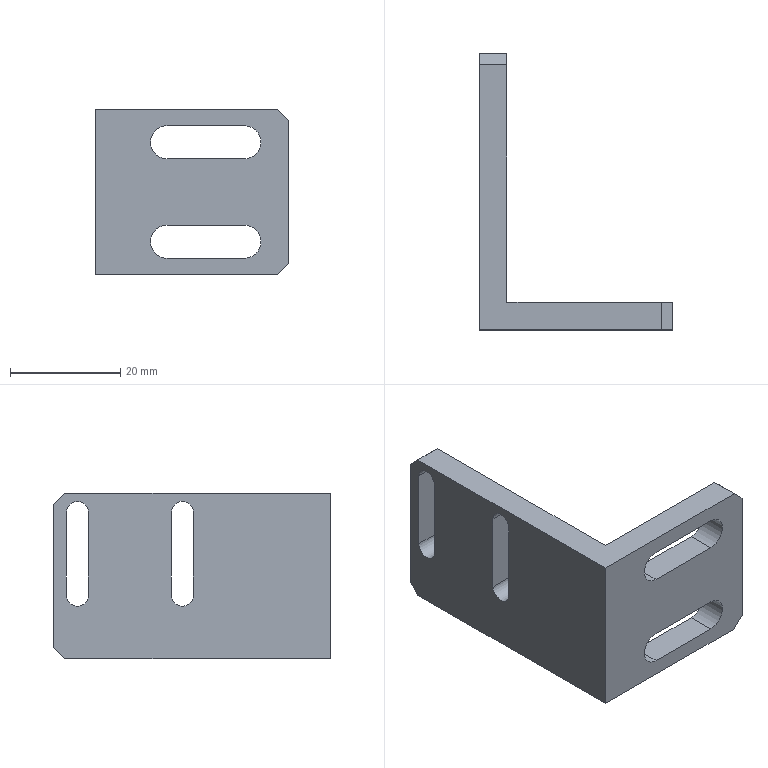Part | STEP file | BB013A02M-04-40A | 1 solid | 30 faces | box 35 x 50 x 30 mm | volume 10112 mm3 | plane 20 | cylinder 10 | commonest cylinder face diameters 6 x6 4 x4